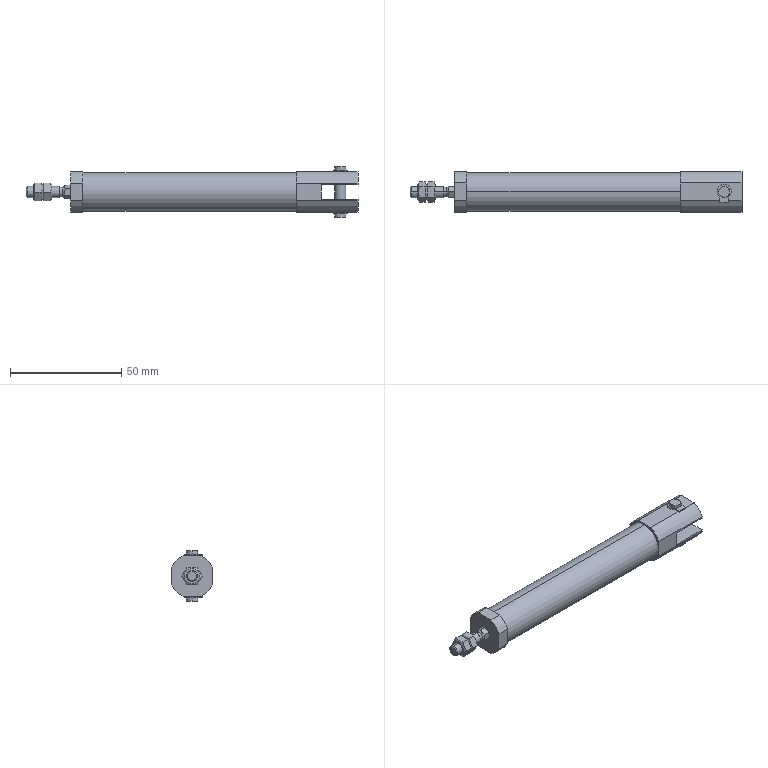Part | STEP file | CJ2KD16-45S_0_0_0_ | 5 solids | 132 faces | box 149 x 18.3 x 22.7 mm | volume 23348 mm3 | plane 57 | cylinder 47 | cone 28 | commonest cylinder face diameters 5 x12 20 x8 4.134 x6 6.4 x6 4.8 x4 16 x4